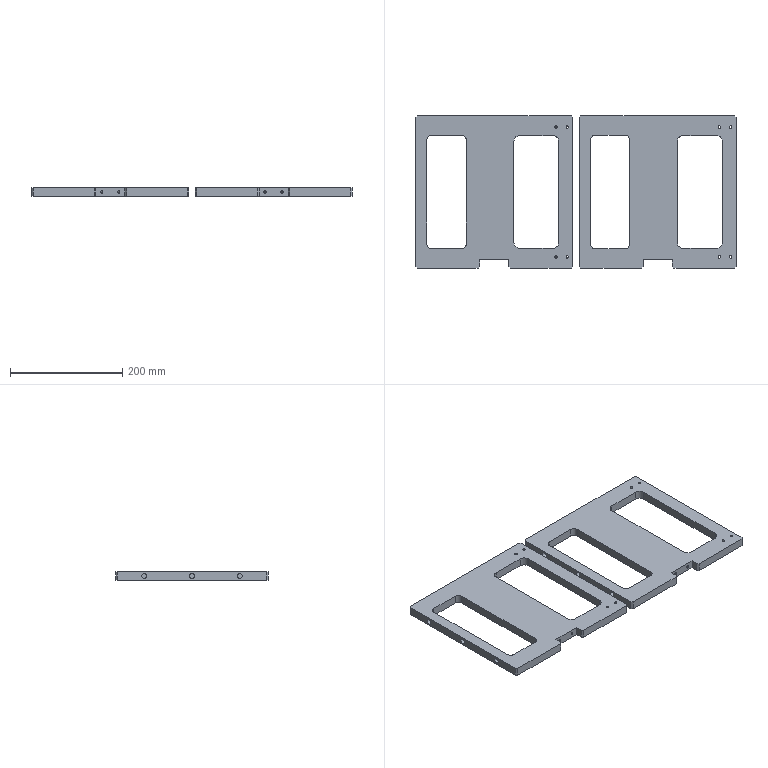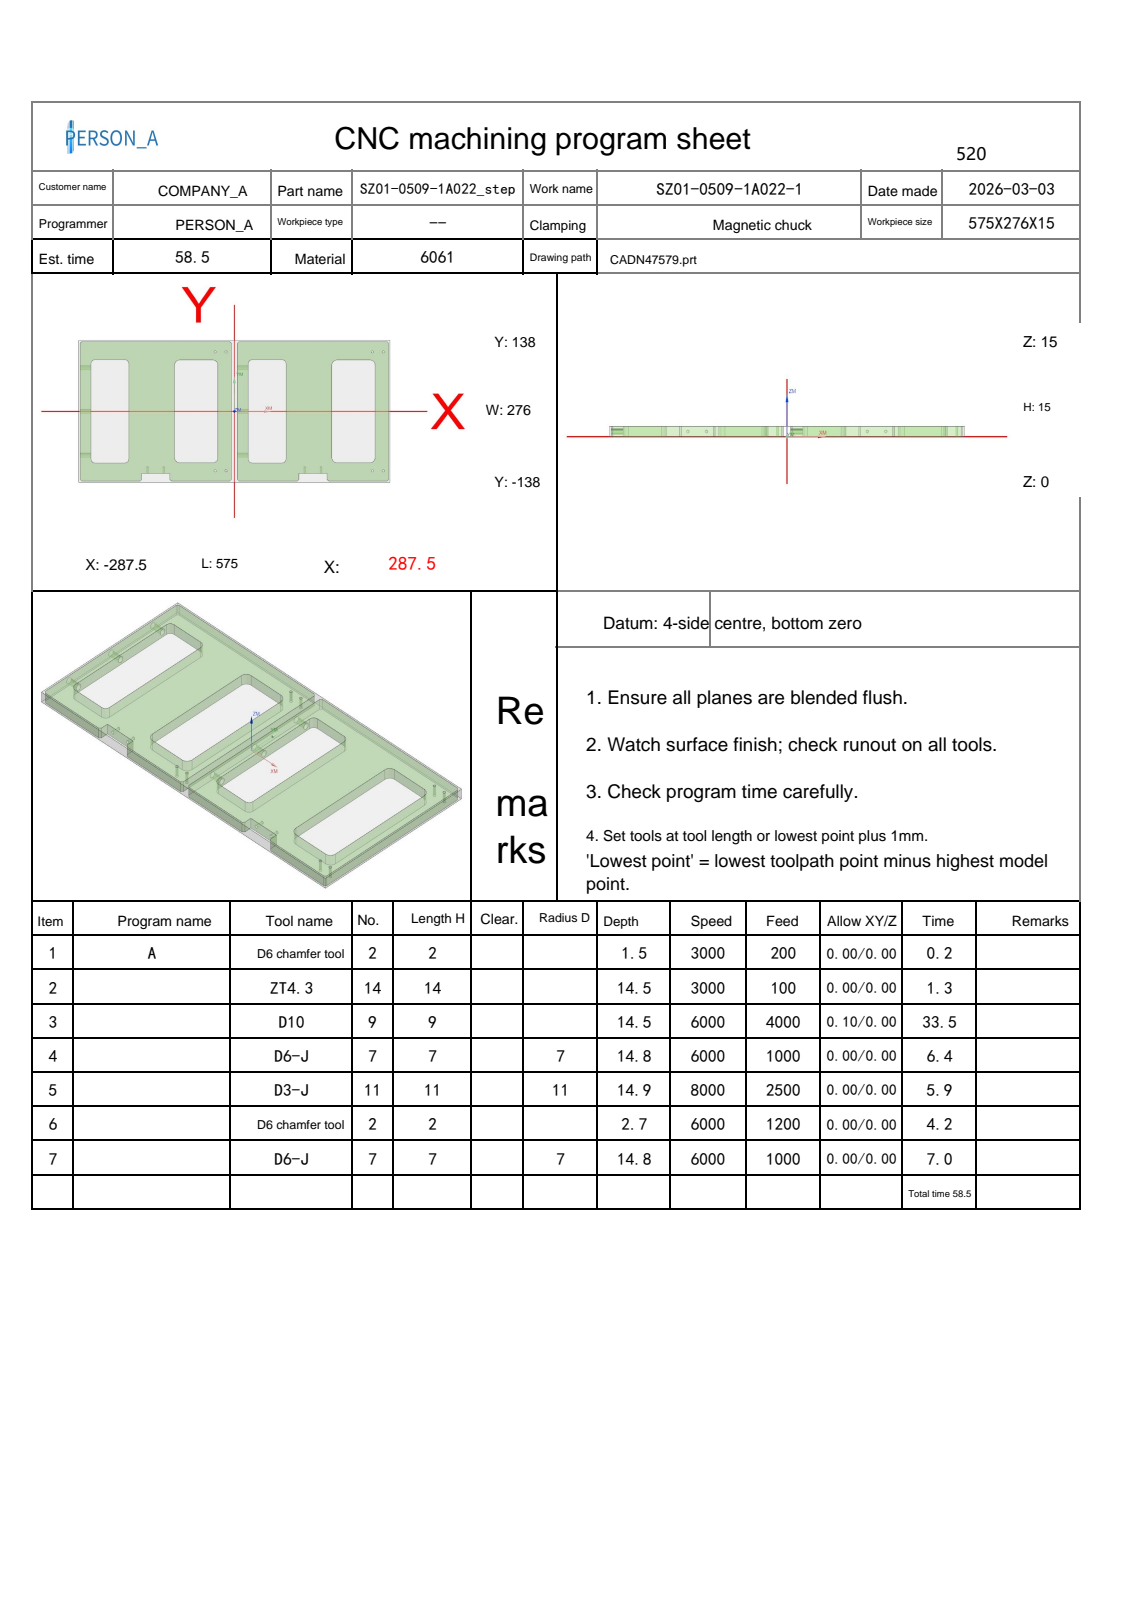NC program | NX | posted by the shop | part box 570 x 271 x 15 mm
Lines 1 to 56 of 10286:
%
O0001
(Machine time: 59.92 MIN)
(===Total Tool:5===)
(T2=D6 chamfer tool   D=6.   R=0.   D-  H02 Z=12.3  )
(T14=ZT4.3  D=4.3  DR_a=118 D-  H14 Z=0.5   )
(T9=D10     D=10.  R=0.   D-  H09 Z=0.5   )
(T7=D6-J    D=6.   R=0.   D7  H07 Z=0.2   )
(T11=D3-J   D=3.   R=0.   D11 H11 Z=0.15  )
G80 G90 G17 G49 G40
G91 G28 Z0
M01
N1 T02 M06
(D6 chamfer tool D=6. R=0. H=02 ce=0.00 di=0.00)
(MAX_Z=45. MIN_Z=13.5 Time=0.17M)
G00 G90 G54 X-15.5 Y115.5 M03 S3000
G43 H02 Z45.
M08
G98 G81 X-15.5 Y115.5 Z13.5 R16. F200.
X-35.5
Y-115.5
X-15.5
X255.
X275.
Y115.5
X255.
G80
G00 Z45.
G91 G28 Z0.0
M05
M09
G91 G28 Z0.0
M01
N2 T14 M06
(ZT4.3 D=4.3 DR_a=118 H=14)
(MAX_Z=45. MIN_Z=0.5 Time=1.32M)
G00 G90 G54 X-15.5 Y115.5 M03 S3000
G43 H14 Z45.
M08
G98 G83 X-15.5 Y115.5 Z.5 R16. F100. Q1.5
X-35.5
Y-115.5
X-15.5
X255.
X275.
Y115.5
X255.
G80
G00 Z45.
G91 G28 Z0.0
M05
M09
G91 G28 Z0.0
M01